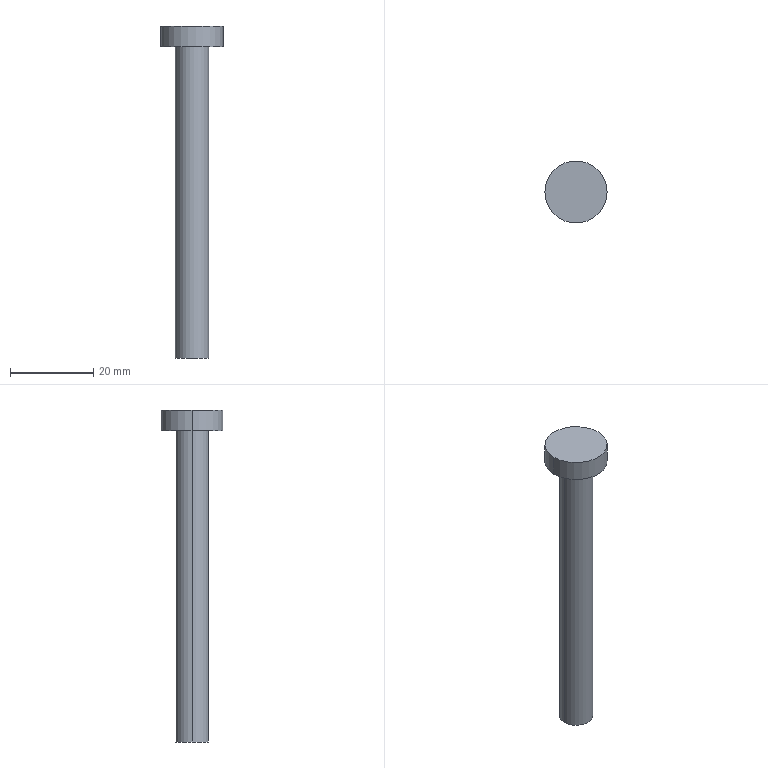Part | SolidWorks | features Extrusion 1, ICE 1 | 1 solid | 7 faces | box 15 x 15 x 80 mm | volume 4653 mm3 | cylinder 4 | plane 3 | commonest cylinder face diameters 8 x2 15 x2
STEP:
#1=CARTESIAN_POINT('',(7.5,0.,80.));
#2=VERTEX_POINT('',#1);
#3=CARTESIAN_POINT('',(-7.5,0.,80.));
#4=VERTEX_POINT('',#3);
#5=CARTESIAN_POINT('',(0.,0.,80.));
#6=DIRECTION('',(0.,0.,1.));
#7=DIRECTION('',(1.,0.,0.));
#8=AXIS2_PLACEMENT_3D('',#5,#6,#7);
#9=CIRCLE('',#8,7.5);
#10=EDGE_CURVE('',#2,#4,#9,.T.);
#11=ORIENTED_EDGE('',*,*,#10,.F.);
#12=CARTESIAN_POINT('',(7.5,0.,75.));
#13=VERTEX_POINT('',#12);
#14=CARTESIAN_POINT('',(7.5,0.,80.));
#15=DIRECTION('',(0.,0.,-1.));
#16=VECTOR('',#15,1000.);
#17=LINE('',#14,#16);
#18=EDGE_CURVE('',#2,#13,#17,.T.);
#19=ORIENTED_EDGE('',*,*,#18,.T.);
#20=CARTESIAN_POINT('',(-7.5,0.,75.));
#21=VERTEX_POINT('',#20);
#22=CARTESIAN_POINT('',(0.,0.,75.));
#23=DIRECTION('',(0.,0.,1.));
#24=DIRECTION('',(1.,0.,0.));
#25=AXIS2_PLACEMENT_3D('',#22,#23,#24);
#26=CIRCLE('',#25,7.5);
#27=EDGE_CURVE('',#13,#21,#26,.T.);
#28=ORIENTED_EDGE('',*,*,#27,.T.);
#29=CARTESIAN_POINT('',(-7.5,0.,80.));
#30=DIRECTION('',(0.,0.,-1.));
#31=VECTOR('',#30,1000.);
#32=LINE('',#29,#31);
#33=EDGE_CURVE('',#4,#21,#32,.T.);
#34=ORIENTED_EDGE('',*,*,#33,.F.);
#35=EDGE_LOOP('',(#11,#19,#28,#34));
#36=FACE_OUTER_BOUND('',#35,.T.);
#37=CARTESIAN_POINT('',(0.,0.,80.));
#38=DIRECTION('',(0.,0.,-1.));
#39=DIRECTION('',(-1.,0.,0.));
#40=AXIS2_PLACEMENT_3D('',#37,#38,#39);
#41=CYLINDRICAL_SURFACE('',#40,7.5);
#42=ADVANCED_FACE('',(#36),#41,.T.);
#43=CARTESIAN_POINT('',(4.,0.,75.));
#44=VERTEX_POINT('',#43);
#45=CARTESIAN_POINT('',(-4.,0.,75.));
#46=VERTEX_POINT('',#45);
#47=CARTESIAN_POINT('',(0.,0.,75.));
#48=DIRECTION('',(0.,0.,1.));
#49=DIRECTION('',(1.,0.,0.));
#50=AXIS2_PLACEMENT_3D('',#47,#48,#49);
#51=CIRCLE('',#50,4.);
#52=EDGE_CURVE('',#44,#46,#51,.T.);
#53=ORIENTED_EDGE('',*,*,#52,.F.);
#54=CARTESIAN_POINT('',(4.,0.,0.));
#55=VERTEX_POINT('',#54);
#56=CARTESIAN_POINT('',(4.,0.,75.));
#57=DIRECTION('',(0.,0.,-1.));
#58=VECTOR('',#57,1000.);
#59=LINE('',#56,#58);
#60=EDGE_CURVE('',#44,#55,#59,.T.);
#61=ORIENTED_EDGE('',*,*,#60,.T.);
#62=CARTESIAN_POINT('',(-4.,0.,0.));
#63=VERTEX_POINT('',#62);
#64=CARTESIAN_POINT('',(0.,0.,0.));
#65=DIRECTION('',(0.,0.,1.));
#66=DIRECTION('',(1.,0.,0.));
#67=AXIS2_PLACEMENT_3D('',#64,#65,#66);
#68=CIRCLE('',#67,4.);
#69=EDGE_CURVE('',#55,#63,#68,.T.);
#70=ORIENTED_EDGE('',*,*,#69,.T.);
#71=CARTESIAN_POINT('',(-4.,0.,75.));
#72=DIRECTION('',(0.,0.,-1.));
#73=VECTOR('',#72,1000.);
#74=LINE('',#71,#73);
#75=EDGE_CURVE('',#46,#63,#74,.T.);
#76=ORIENTED_EDGE('',*,*,#75,.F.);
#77=EDGE_LOOP('',(#53,#61,#70,#76));
#78=FACE_OUTER_BOUND('',#77,.T.);
#79=CARTESIAN_POINT('',(0.,0.,75.));
#80=DIRECTION('',(0.,0.,-1.));
#81=DIRECTION('',(-1.,0.,0.));
#82=AXIS2_PLACEMENT_3D('',#79,#80,#81);
#83=CYLINDRICAL_SURFACE('',#82,4.);
#84=ADVANCED_FACE('',(#78),#83,.T.);
#85=ORIENTED_EDGE('',*,*,#60,.F.);
#86=CARTESIAN_POINT('',(0.,0.,75.));
#87=DIRECTION('',(0.,0.,1.));
#88=DIRECTION('',(1.,0.,0.));
#89=AXIS2_PLACEMENT_3D('',#86,#87,#88);
#90=CIRCLE('',#89,4.);
#91=EDGE_CURVE('',#46,#44,#90,.T.);
#92=ORIENTED_EDGE('',*,*,#91,.F.);
#93=ORIENTED_EDGE('',*,*,#75,.T.);
#94=CARTESIAN_POINT('',(0.,0.,0.));
#95=DIRECTION('',(0.,0.,1.));
#96=DIRECTION('',(1.,0.,0.));
#97=AXIS2_PLACEMENT_3D('',#94,#95,#96);
#98=CIRCLE('',#97,4.);
#99=EDGE_CURVE('',#63,#55,#98,.T.);
#100=ORIENTED_EDGE('',*,*,#99,.T.);
#101=EDGE_LOOP('',(#85,#92,#93,#100));
#102=FACE_OUTER_BOUND('',#101,.T.);
#103=CARTESIAN_POINT('',(0.,0.,75.));
#104=DIRECTION('',(0.,0.,-1.));
#105=DIRECTION('',(-1.,0.,0.));
#106=AXIS2_PLACEMENT_3D('',#103,#104,#105);
#107=CYLINDRICAL_SURFACE('',#106,4.);
#108=ADVANCED_FACE('',(#102),#107,.T.);
#109=ORIENTED_EDGE('',*,*,#99,.F.);
#110=ORIENTED_EDGE('',*,*,#69,.F.);
#111=EDGE_LOOP('',(#109,#110));
#112=FACE_OUTER_BOUND('',#111,.T.);
#113=CARTESIAN_POINT('',(0.,0.,0.));
#114=DIRECTION('',(0.,0.,1.));
#115=DIRECTION('',(1.,0.,0.));
#116=AXIS2_PLACEMENT_3D('',#113,#114,#115);
#117=PLANE('',#116);
#118=ADVANCED_FACE('',(#112),#117,.F.);
#119=ORIENTED_EDGE('',*,*,#18,.F.);
#120=CARTESIAN_POINT('',(0.,0.,80.));
#121=DIRECTION('',(0.,0.,1.));
#122=DIRECTION('',(1.,0.,0.));
#123=AXIS2_PLACEMENT_3D('',#120,#121,#122);
#124=CIRCLE('',#123,7.5);
#125=EDGE_CURVE('',#4,#2,#124,.T.);
#126=ORIENTED_EDGE('',*,*,#125,.F.);
#127=ORIENTED_EDGE('',*,*,#33,.T.);
#128=CARTESIAN_POINT('',(0.,0.,75.));
#129=DIRECTION('',(0.,0.,1.));
#130=DIRECTION('',(1.,0.,0.));
#131=AXIS2_PLACEMENT_3D('',#128,#129,#130);
#132=CIRCLE('',#131,7.5);
#133=EDGE_CURVE('',#21,#13,#132,.T.);
#134=ORIENTED_EDGE('',*,*,#133,.T.);
#135=EDGE_LOOP('',(#119,#126,#127,#134));
#136=FACE_OUTER_BOUND('',#135,.T.);
#137=CARTESIAN_POINT('',(0.,0.,80.));
#138=DIRECTION('',(0.,0.,-1.));
#139=DIRECTION('',(-1.,0.,0.));
#140=AXIS2_PLACEMENT_3D('',#137,#138,#139);
#141=CYLINDRICAL_SURFACE('',#140,7.5);
#142=ADVANCED_FACE('',(#136),#141,.T.);
#143=ORIENTED_EDGE('',*,*,#125,.T.);
#144=ORIENTED_EDGE('',*,*,#10,.T.);
#145=EDGE_LOOP('',(#143,#144));
#146=FACE_OUTER_BOUND('',#145,.T.);
#147=CARTESIAN_POINT('',(0.,0.,80.));
#148=DIRECTION('',(0.,0.,1.));
#149=DIRECTION('',(1.,0.,0.));
#150=AXIS2_PLACEMENT_3D('',#147,#148,#149);
#151=PLANE('',#150);
#152=ADVANCED_FACE('',(#146),#151,.T.);
#153=ORIENTED_EDGE('',*,*,#91,.T.);
#154=ORIENTED_EDGE('',*,*,#52,.T.);
#155=EDGE_LOOP('',(#153,#154));
#156=FACE_BOUND('',#155,.T.);
#157=ORIENTED_EDGE('',*,*,#133,.F.);
#158=ORIENTED_EDGE('',*,*,#27,.F.);
#159=EDGE_LOOP('',(#157,#158));
#160=FACE_OUTER_BOUND('',#159,.T.);
#161=CARTESIAN_POINT('',(0.,0.,75.));
#162=DIRECTION('',(0.,0.,1.));
#163=DIRECTION('',(1.,0.,0.));
#164=AXIS2_PLACEMENT_3D('',#161,#162,#163);
#165=PLANE('',#164);
#166=ADVANCED_FACE('',(#156,#160),#165,.F.);
#167=CLOSED_SHELL('',(#42,#84,#108,#118,#142,#152,#166));
#168=MANIFOLD_SOLID_BREP('',#167);
#169=CARTESIAN_POINT('',(0.,0.,0.));
#170=DIRECTION('',(0.,0.,1.));
#171=DIRECTION('',(1.,0.,0.));
#172=AXIS2_PLACEMENT_3D('',#169,#170,#171);
#173=(LENGTH_UNIT()NAMED_UNIT(*)SI_UNIT(.MILLI.,.METRE.));
#174=UNCERTAINTY_MEASURE_WITH_UNIT(LENGTH_MEASURE(0.00001),#173,'','');
#175=(NAMED_UNIT(*)PLANE_ANGLE_UNIT()SI_UNIT($,.RADIAN.));
#176=(NAMED_UNIT(*)SI_UNIT($,.STERADIAN.)SOLID_ANGLE_UNIT());
#177=(GEOMETRIC_REPRESENTATION_CONTEXT(3)GLOBAL_UNCERTAINTY_ASSIGNED_CONTEXT((#174))GLOBAL_UNIT_ASSIGNED_CONTEXT((#173,#175,#176))REPRESENTATION_CONTEXT('',''));
#178=ADVANCED_BREP_SHAPE_REPRESENTATION('',(#168,#172),#177);